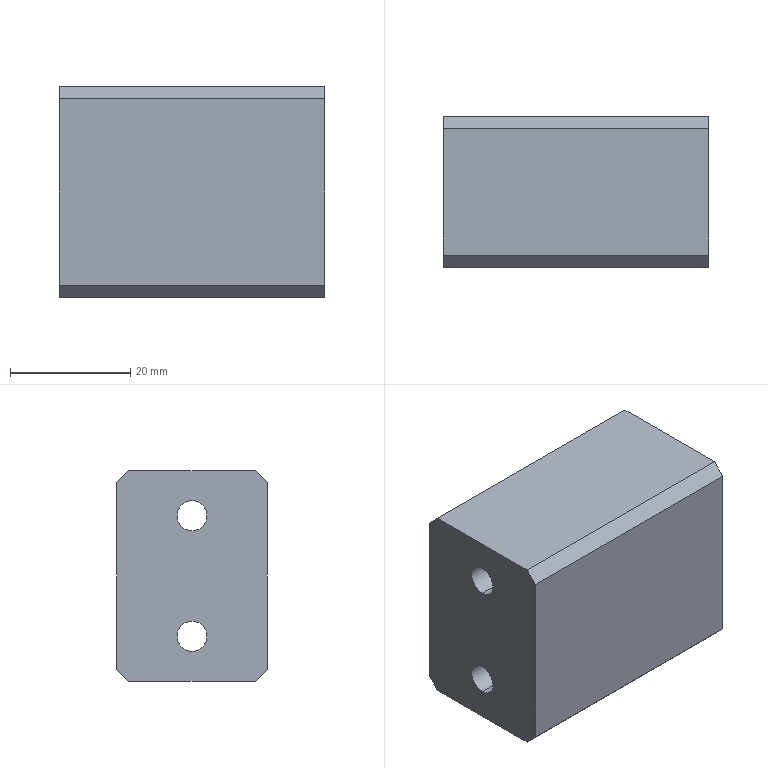Part | SolidWorks | features BaseBody 1 | 1 solid | 14 faces | box 44 x 25 x 35 mm | volume 36420 mm3 | plane 10 | cylinder 4 | commonest cylinder face diameters 5 x4
STEP:
#1=CARTESIAN_POINT('',(35.247,1517.,-337.));
#2=VERTEX_POINT('',#1);
#3=CARTESIAN_POINT('',(35.247,1517.,-332.));
#4=VERTEX_POINT('',#3);
#5=CARTESIAN_POINT('',(35.247,1517.,-334.5));
#6=DIRECTION('',(-1.,0.,0.));
#7=DIRECTION('',(0.,0.,-1.));
#8=AXIS2_PLACEMENT_3D('',#5,#6,#7);
#9=CIRCLE('',#8,2.5);
#10=EDGE_CURVE('',#2,#4,#9,.T.);
#11=ORIENTED_EDGE('',*,*,#10,.T.);
#12=CARTESIAN_POINT('',(79.247,1517.,-332.));
#13=VERTEX_POINT('',#12);
#14=CARTESIAN_POINT('',(79.247,1517.,-332.));
#15=DIRECTION('',(1.,0.,0.));
#16=VECTOR('',#15,1000.);
#17=LINE('',#14,#16);
#18=EDGE_CURVE('',#4,#13,#17,.T.);
#19=ORIENTED_EDGE('',*,*,#18,.T.);
#20=CARTESIAN_POINT('',(79.247,1517.,-337.));
#21=VERTEX_POINT('',#20);
#22=CARTESIAN_POINT('',(79.247,1517.,-334.5));
#23=DIRECTION('',(-1.,0.,0.));
#24=DIRECTION('',(0.,0.,-1.));
#25=AXIS2_PLACEMENT_3D('',#22,#23,#24);
#26=CIRCLE('',#25,2.5);
#27=EDGE_CURVE('',#21,#13,#26,.T.);
#28=ORIENTED_EDGE('',*,*,#27,.F.);
#29=CARTESIAN_POINT('',(79.247,1517.,-337.));
#30=DIRECTION('',(1.,0.,0.));
#31=VECTOR('',#30,1000.);
#32=LINE('',#29,#31);
#33=EDGE_CURVE('',#2,#21,#32,.T.);
#34=ORIENTED_EDGE('',*,*,#33,.F.);
#35=EDGE_LOOP('',(#11,#19,#28,#34));
#36=FACE_OUTER_BOUND('',#35,.T.);
#37=CARTESIAN_POINT('',(79.247,1517.,-334.5));
#38=DIRECTION('',(1.,0.,0.));
#39=DIRECTION('',(0.,0.,-1.));
#40=AXIS2_PLACEMENT_3D('',#37,#38,#39);
#41=CYLINDRICAL_SURFACE('',#40,2.5);
#42=ADVANCED_FACE('',(#36),#41,.F.);
#43=CARTESIAN_POINT('',(35.247,1517.,-357.));
#44=VERTEX_POINT('',#43);
#45=CARTESIAN_POINT('',(35.247,1517.,-352.));
#46=VERTEX_POINT('',#45);
#47=CARTESIAN_POINT('',(35.247,1517.,-354.5));
#48=DIRECTION('',(-1.,0.,0.));
#49=DIRECTION('',(0.,0.,-1.));
#50=AXIS2_PLACEMENT_3D('',#47,#48,#49);
#51=CIRCLE('',#50,2.5);
#52=EDGE_CURVE('',#44,#46,#51,.T.);
#53=ORIENTED_EDGE('',*,*,#52,.T.);
#54=CARTESIAN_POINT('',(79.247,1517.,-352.));
#55=VERTEX_POINT('',#54);
#56=CARTESIAN_POINT('',(79.247,1517.,-352.));
#57=DIRECTION('',(1.,0.,0.));
#58=VECTOR('',#57,1000.);
#59=LINE('',#56,#58);
#60=EDGE_CURVE('',#46,#55,#59,.T.);
#61=ORIENTED_EDGE('',*,*,#60,.T.);
#62=CARTESIAN_POINT('',(79.247,1517.,-357.));
#63=VERTEX_POINT('',#62);
#64=CARTESIAN_POINT('',(79.247,1517.,-354.5));
#65=DIRECTION('',(-1.,0.,0.));
#66=DIRECTION('',(0.,0.,-1.));
#67=AXIS2_PLACEMENT_3D('',#64,#65,#66);
#68=CIRCLE('',#67,2.5);
#69=EDGE_CURVE('',#63,#55,#68,.T.);
#70=ORIENTED_EDGE('',*,*,#69,.F.);
#71=CARTESIAN_POINT('',(79.247,1517.,-357.));
#72=DIRECTION('',(1.,0.,0.));
#73=VECTOR('',#72,1000.);
#74=LINE('',#71,#73);
#75=EDGE_CURVE('',#44,#63,#74,.T.);
#76=ORIENTED_EDGE('',*,*,#75,.F.);
#77=EDGE_LOOP('',(#53,#61,#70,#76));
#78=FACE_OUTER_BOUND('',#77,.T.);
#79=CARTESIAN_POINT('',(79.247,1517.,-354.5));
#80=DIRECTION('',(1.,0.,0.));
#81=DIRECTION('',(0.,0.,-1.));
#82=AXIS2_PLACEMENT_3D('',#79,#80,#81);
#83=CYLINDRICAL_SURFACE('',#82,2.5);
#84=ADVANCED_FACE('',(#78),#83,.F.);
#85=CARTESIAN_POINT('',(35.247,1529.5,-329.));
#86=VERTEX_POINT('',#85);
#87=CARTESIAN_POINT('',(35.247,1529.5,-360.));
#88=VERTEX_POINT('',#87);
#89=CARTESIAN_POINT('',(35.247,1529.5,-327.));
#90=DIRECTION('',(0.,0.,-1.));
#91=VECTOR('',#90,1000.);
#92=LINE('',#89,#91);
#93=EDGE_CURVE('',#86,#88,#92,.T.);
#94=ORIENTED_EDGE('',*,*,#93,.F.);
#95=CARTESIAN_POINT('',(79.247,1529.5,-329.));
#96=VERTEX_POINT('',#95);
#97=CARTESIAN_POINT('',(79.247,1529.5,-329.));
#98=DIRECTION('',(-1.,0.,0.));
#99=VECTOR('',#98,1000.);
#100=LINE('',#97,#99);
#101=EDGE_CURVE('',#96,#86,#100,.T.);
#102=ORIENTED_EDGE('',*,*,#101,.F.);
#103=CARTESIAN_POINT('',(79.247,1529.5,-360.));
#104=VERTEX_POINT('',#103);
#105=CARTESIAN_POINT('',(79.247,1529.5,-327.));
#106=DIRECTION('',(0.,0.,1.));
#107=VECTOR('',#106,1000.);
#108=LINE('',#105,#107);
#109=EDGE_CURVE('',#104,#96,#108,.T.);
#110=ORIENTED_EDGE('',*,*,#109,.F.);
#111=CARTESIAN_POINT('',(79.247,1529.5,-360.));
#112=DIRECTION('',(1.,0.,0.));
#113=VECTOR('',#112,1000.);
#114=LINE('',#111,#113);
#115=EDGE_CURVE('',#88,#104,#114,.T.);
#116=ORIENTED_EDGE('',*,*,#115,.F.);
#117=EDGE_LOOP('',(#94,#102,#110,#116));
#118=FACE_OUTER_BOUND('',#117,.T.);
#119=CARTESIAN_POINT('',(79.247,1529.5,-327.));
#120=DIRECTION('',(0.,-1.,0.));
#121=DIRECTION('',(0.,0.,-1.));
#122=AXIS2_PLACEMENT_3D('',#119,#120,#121);
#123=PLANE('',#122);
#124=ADVANCED_FACE('',(#118),#123,.F.);
#125=CARTESIAN_POINT('',(35.247,1527.5,-362.));
#126=VERTEX_POINT('',#125);
#127=CARTESIAN_POINT('',(35.247,1529.5,-360.));
#128=DIRECTION('',(0.,-0.7071,-0.7071));
#129=VECTOR('',#128,1000.);
#130=LINE('',#127,#129);
#131=EDGE_CURVE('',#88,#126,#130,.T.);
#132=ORIENTED_EDGE('',*,*,#131,.F.);
#133=ORIENTED_EDGE('',*,*,#115,.T.);
#134=CARTESIAN_POINT('',(79.247,1527.5,-362.));
#135=VERTEX_POINT('',#134);
#136=CARTESIAN_POINT('',(79.247,1529.5,-360.));
#137=DIRECTION('',(0.,0.7071,0.7071));
#138=VECTOR('',#137,1000.);
#139=LINE('',#136,#138);
#140=EDGE_CURVE('',#135,#104,#139,.T.);
#141=ORIENTED_EDGE('',*,*,#140,.F.);
#142=CARTESIAN_POINT('',(79.247,1527.5,-362.));
#143=DIRECTION('',(1.,0.,0.));
#144=VECTOR('',#143,1000.);
#145=LINE('',#142,#144);
#146=EDGE_CURVE('',#126,#135,#145,.T.);
#147=ORIENTED_EDGE('',*,*,#146,.F.);
#148=EDGE_LOOP('',(#132,#133,#141,#147));
#149=FACE_OUTER_BOUND('',#148,.T.);
#150=CARTESIAN_POINT('',(79.247,1529.5,-360.));
#151=DIRECTION('',(0.,-0.7071,0.7071));
#152=DIRECTION('',(0.,-0.7071,-0.7071));
#153=AXIS2_PLACEMENT_3D('',#150,#151,#152);
#154=PLANE('',#153);
#155=ADVANCED_FACE('',(#149),#154,.F.);
#156=ORIENTED_EDGE('',*,*,#10,.F.);
#157=CARTESIAN_POINT('',(35.247,1517.,-334.5));
#158=DIRECTION('',(-1.,0.,0.));
#159=DIRECTION('',(0.,0.,-1.));
#160=AXIS2_PLACEMENT_3D('',#157,#158,#159);
#161=CIRCLE('',#160,2.5);
#162=EDGE_CURVE('',#4,#2,#161,.T.);
#163=ORIENTED_EDGE('',*,*,#162,.F.);
#164=EDGE_LOOP('',(#156,#163));
#165=FACE_BOUND('',#164,.T.);
#166=ORIENTED_EDGE('',*,*,#52,.F.);
#167=CARTESIAN_POINT('',(35.247,1517.,-354.5));
#168=DIRECTION('',(-1.,0.,0.));
#169=DIRECTION('',(0.,0.,-1.));
#170=AXIS2_PLACEMENT_3D('',#167,#168,#169);
#171=CIRCLE('',#170,2.5);
#172=EDGE_CURVE('',#46,#44,#171,.T.);
#173=ORIENTED_EDGE('',*,*,#172,.F.);
#174=EDGE_LOOP('',(#166,#173));
#175=FACE_BOUND('',#174,.T.);
#176=CARTESIAN_POINT('',(35.247,1506.5,-362.));
#177=VERTEX_POINT('',#176);
#178=CARTESIAN_POINT('',(35.247,1517.,-362.));
#179=DIRECTION('',(0.,1.,0.));
#180=VECTOR('',#179,1000.);
#181=LINE('',#178,#180);
#182=EDGE_CURVE('',#177,#126,#181,.T.);
#183=ORIENTED_EDGE('',*,*,#182,.F.);
#184=CARTESIAN_POINT('',(35.247,1504.5,-360.));
#185=VERTEX_POINT('',#184);
#186=CARTESIAN_POINT('',(35.247,1504.5,-360.));
#187=DIRECTION('',(0.,0.7071,-0.7071));
#188=VECTOR('',#187,1000.);
#189=LINE('',#186,#188);
#190=EDGE_CURVE('',#185,#177,#189,.T.);
#191=ORIENTED_EDGE('',*,*,#190,.F.);
#192=CARTESIAN_POINT('',(35.247,1504.5,-329.));
#193=VERTEX_POINT('',#192);
#194=CARTESIAN_POINT('',(35.247,1504.5,-344.5));
#195=DIRECTION('',(0.,0.,-1.));
#196=VECTOR('',#195,1000.);
#197=LINE('',#194,#196);
#198=EDGE_CURVE('',#193,#185,#197,.T.);
#199=ORIENTED_EDGE('',*,*,#198,.F.);
#200=CARTESIAN_POINT('',(35.247,1506.5,-327.));
#201=VERTEX_POINT('',#200);
#202=CARTESIAN_POINT('',(35.247,1506.5,-327.));
#203=DIRECTION('',(0.,-0.7071,-0.7071));
#204=VECTOR('',#203,1000.);
#205=LINE('',#202,#204);
#206=EDGE_CURVE('',#201,#193,#205,.T.);
#207=ORIENTED_EDGE('',*,*,#206,.F.);
#208=CARTESIAN_POINT('',(35.247,1527.5,-327.));
#209=VERTEX_POINT('',#208);
#210=CARTESIAN_POINT('',(35.247,1517.,-327.));
#211=DIRECTION('',(0.,-1.,0.));
#212=VECTOR('',#211,1000.);
#213=LINE('',#210,#212);
#214=EDGE_CURVE('',#209,#201,#213,.T.);
#215=ORIENTED_EDGE('',*,*,#214,.F.);
#216=CARTESIAN_POINT('',(35.247,1529.5,-329.));
#217=DIRECTION('',(0.,-0.7071,0.7071));
#218=VECTOR('',#217,1000.);
#219=LINE('',#216,#218);
#220=EDGE_CURVE('',#86,#209,#219,.T.);
#221=ORIENTED_EDGE('',*,*,#220,.F.);
#222=ORIENTED_EDGE('',*,*,#93,.T.);
#223=ORIENTED_EDGE('',*,*,#131,.T.);
#224=EDGE_LOOP('',(#183,#191,#199,#207,#215,#221,#222,#223));
#225=FACE_OUTER_BOUND('',#224,.T.);
#226=CARTESIAN_POINT('',(35.247,1517.,-344.5));
#227=DIRECTION('',(1.,0.,0.));
#228=DIRECTION('',(0.,0.,-1.));
#229=AXIS2_PLACEMENT_3D('',#226,#227,#228);
#230=PLANE('',#229);
#231=ADVANCED_FACE('',(#165,#175,#225),#230,.F.);
#232=ORIENTED_EDGE('',*,*,#220,.T.);
#233=CARTESIAN_POINT('',(79.247,1527.5,-327.));
#234=VERTEX_POINT('',#233);
#235=CARTESIAN_POINT('',(79.247,1527.5,-327.));
#236=DIRECTION('',(-1.,0.,0.));
#237=VECTOR('',#236,1000.);
#238=LINE('',#235,#237);
#239=EDGE_CURVE('',#234,#209,#238,.T.);
#240=ORIENTED_EDGE('',*,*,#239,.F.);
#241=CARTESIAN_POINT('',(79.247,1527.5,-327.));
#242=DIRECTION('',(0.,-0.7071,0.7071));
#243=VECTOR('',#242,1000.);
#244=LINE('',#241,#243);
#245=EDGE_CURVE('',#96,#234,#244,.T.);
#246=ORIENTED_EDGE('',*,*,#245,.F.);
#247=ORIENTED_EDGE('',*,*,#101,.T.);
#248=EDGE_LOOP('',(#232,#240,#246,#247));
#249=FACE_OUTER_BOUND('',#248,.T.);
#250=CARTESIAN_POINT('',(79.247,1527.5,-327.));
#251=DIRECTION('',(0.,-0.7071,-0.7071));
#252=DIRECTION('',(0.,0.7071,-0.7071));
#253=AXIS2_PLACEMENT_3D('',#250,#251,#252);
#254=PLANE('',#253);
#255=ADVANCED_FACE('',(#249),#254,.F.);
#256=ORIENTED_EDGE('',*,*,#27,.T.);
#257=CARTESIAN_POINT('',(79.247,1517.,-334.5));
#258=DIRECTION('',(-1.,0.,0.));
#259=DIRECTION('',(0.,0.,-1.));
#260=AXIS2_PLACEMENT_3D('',#257,#258,#259);
#261=CIRCLE('',#260,2.5);
#262=EDGE_CURVE('',#13,#21,#261,.T.);
#263=ORIENTED_EDGE('',*,*,#262,.T.);
#264=EDGE_LOOP('',(#256,#263));
#265=FACE_BOUND('',#264,.T.);
#266=ORIENTED_EDGE('',*,*,#69,.T.);
#267=CARTESIAN_POINT('',(79.247,1517.,-354.5));
#268=DIRECTION('',(-1.,0.,0.));
#269=DIRECTION('',(0.,0.,-1.));
#270=AXIS2_PLACEMENT_3D('',#267,#268,#269);
#271=CIRCLE('',#270,2.5);
#272=EDGE_CURVE('',#55,#63,#271,.T.);
#273=ORIENTED_EDGE('',*,*,#272,.T.);
#274=EDGE_LOOP('',(#266,#273));
#275=FACE_BOUND('',#274,.T.);
#276=CARTESIAN_POINT('',(79.247,1504.5,-360.));
#277=VERTEX_POINT('',#276);
#278=CARTESIAN_POINT('',(79.247,1506.5,-362.));
#279=VERTEX_POINT('',#278);
#280=CARTESIAN_POINT('',(79.247,1504.5,-360.));
#281=DIRECTION('',(0.,0.7071,-0.7071));
#282=VECTOR('',#281,1000.);
#283=LINE('',#280,#282);
#284=EDGE_CURVE('',#277,#279,#283,.T.);
#285=ORIENTED_EDGE('',*,*,#284,.T.);
#286=CARTESIAN_POINT('',(79.247,1517.,-362.));
#287=DIRECTION('',(0.,1.,0.));
#288=VECTOR('',#287,1000.);
#289=LINE('',#286,#288);
#290=EDGE_CURVE('',#279,#135,#289,.T.);
#291=ORIENTED_EDGE('',*,*,#290,.T.);
#292=ORIENTED_EDGE('',*,*,#140,.T.);
#293=ORIENTED_EDGE('',*,*,#109,.T.);
#294=ORIENTED_EDGE('',*,*,#245,.T.);
#295=CARTESIAN_POINT('',(79.247,1506.5,-327.));
#296=VERTEX_POINT('',#295);
#297=CARTESIAN_POINT('',(79.247,1517.,-327.));
#298=DIRECTION('',(0.,-1.,0.));
#299=VECTOR('',#298,1000.);
#300=LINE('',#297,#299);
#301=EDGE_CURVE('',#234,#296,#300,.T.);
#302=ORIENTED_EDGE('',*,*,#301,.T.);
#303=CARTESIAN_POINT('',(79.247,1504.5,-329.));
#304=VERTEX_POINT('',#303);
#305=CARTESIAN_POINT('',(79.247,1506.5,-327.));
#306=DIRECTION('',(0.,-0.7071,-0.7071));
#307=VECTOR('',#306,1000.);
#308=LINE('',#305,#307);
#309=EDGE_CURVE('',#296,#304,#308,.T.);
#310=ORIENTED_EDGE('',*,*,#309,.T.);
#311=CARTESIAN_POINT('',(79.247,1504.5,-344.5));
#312=DIRECTION('',(0.,0.,-1.));
#313=VECTOR('',#312,1000.);
#314=LINE('',#311,#313);
#315=EDGE_CURVE('',#304,#277,#314,.T.);
#316=ORIENTED_EDGE('',*,*,#315,.T.);
#317=EDGE_LOOP('',(#285,#291,#292,#293,#294,#302,#310,#316));
#318=FACE_OUTER_BOUND('',#317,.T.);
#319=CARTESIAN_POINT('',(79.247,1517.,-344.5));
#320=DIRECTION('',(1.,0.,0.));
#321=DIRECTION('',(0.,0.,-1.));
#322=AXIS2_PLACEMENT_3D('',#319,#320,#321);
#323=PLANE('',#322);
#324=ADVANCED_FACE('',(#265,#275,#318),#323,.T.);
#325=ORIENTED_EDGE('',*,*,#290,.F.);
#326=CARTESIAN_POINT('',(79.247,1506.5,-362.));
#327=DIRECTION('',(1.,0.,0.));
#328=VECTOR('',#327,1000.);
#329=LINE('',#326,#328);
#330=EDGE_CURVE('',#177,#279,#329,.T.);
#331=ORIENTED_EDGE('',*,*,#330,.F.);
#332=ORIENTED_EDGE('',*,*,#182,.T.);
#333=ORIENTED_EDGE('',*,*,#146,.T.);
#334=EDGE_LOOP('',(#325,#331,#332,#333));
#335=FACE_OUTER_BOUND('',#334,.T.);
#336=CARTESIAN_POINT('',(79.247,1504.5,-362.));
#337=DIRECTION('',(0.,0.,1.));
#338=DIRECTION('',(1.,0.,0.));
#339=AXIS2_PLACEMENT_3D('',#336,#337,#338);
#340=PLANE('',#339);
#341=ADVANCED_FACE('',(#335),#340,.F.);
#342=ORIENTED_EDGE('',*,*,#18,.F.);
#343=ORIENTED_EDGE('',*,*,#162,.T.);
#344=ORIENTED_EDGE('',*,*,#33,.T.);
#345=ORIENTED_EDGE('',*,*,#262,.F.);
#346=EDGE_LOOP('',(#342,#343,#344,#345));
#347=FACE_OUTER_BOUND('',#346,.T.);
#348=CARTESIAN_POINT('',(79.247,1517.,-334.5));
#349=DIRECTION('',(1.,0.,0.));
#350=DIRECTION('',(0.,0.,-1.));
#351=AXIS2_PLACEMENT_3D('',#348,#349,#350);
#352=CYLINDRICAL_SURFACE('',#351,2.5);
#353=ADVANCED_FACE('',(#347),#352,.F.);
#354=ORIENTED_EDGE('',*,*,#60,.F.);
#355=ORIENTED_EDGE('',*,*,#172,.T.);
#356=ORIENTED_EDGE('',*,*,#75,.T.);
#357=ORIENTED_EDGE('',*,*,#272,.F.);
#358=EDGE_LOOP('',(#354,#355,#356,#357));
#359=FACE_OUTER_BOUND('',#358,.T.);
#360=CARTESIAN_POINT('',(79.247,1517.,-354.5));
#361=DIRECTION('',(1.,0.,0.));
#362=DIRECTION('',(0.,0.,-1.));
#363=AXIS2_PLACEMENT_3D('',#360,#361,#362);
#364=CYLINDRICAL_SURFACE('',#363,2.5);
#365=ADVANCED_FACE('',(#359),#364,.F.);
#366=ORIENTED_EDGE('',*,*,#190,.T.);
#367=ORIENTED_EDGE('',*,*,#330,.T.);
#368=ORIENTED_EDGE('',*,*,#284,.F.);
#369=CARTESIAN_POINT('',(79.247,1504.5,-360.));
#370=DIRECTION('',(1.,0.,0.));
#371=VECTOR('',#370,1000.);
#372=LINE('',#369,#371);
#373=EDGE_CURVE('',#185,#277,#372,.T.);
#374=ORIENTED_EDGE('',*,*,#373,.F.);
#375=EDGE_LOOP('',(#366,#367,#368,#374));
#376=FACE_OUTER_BOUND('',#375,.T.);
#377=CARTESIAN_POINT('',(79.247,1506.5,-362.));
#378=DIRECTION('',(0.,0.7071,0.7071));
#379=DIRECTION('',(0.,-0.7071,0.7071));
#380=AXIS2_PLACEMENT_3D('',#377,#378,#379);
#381=PLANE('',#380);
#382=ADVANCED_FACE('',(#376),#381,.F.);
#383=ORIENTED_EDGE('',*,*,#315,.F.);
#384=CARTESIAN_POINT('',(79.247,1504.5,-329.));
#385=DIRECTION('',(1.,0.,0.));
#386=VECTOR('',#385,1000.);
#387=LINE('',#384,#386);
#388=EDGE_CURVE('',#193,#304,#387,.T.);
#389=ORIENTED_EDGE('',*,*,#388,.F.);
#390=ORIENTED_EDGE('',*,*,#198,.T.);
#391=ORIENTED_EDGE('',*,*,#373,.T.);
#392=EDGE_LOOP('',(#383,#389,#390,#391));
#393=FACE_OUTER_BOUND('',#392,.T.);
#394=CARTESIAN_POINT('',(79.247,1504.5,-327.));
#395=DIRECTION('',(0.,1.,0.));
#396=DIRECTION('',(0.,0.,1.));
#397=AXIS2_PLACEMENT_3D('',#394,#395,#396);
#398=PLANE('',#397);
#399=ADVANCED_FACE('',(#393),#398,.F.);
#400=ORIENTED_EDGE('',*,*,#206,.T.);
#401=ORIENTED_EDGE('',*,*,#388,.T.);
#402=ORIENTED_EDGE('',*,*,#309,.F.);
#403=CARTESIAN_POINT('',(79.247,1506.5,-327.));
#404=DIRECTION('',(1.,0.,0.));
#405=VECTOR('',#404,1000.);
#406=LINE('',#403,#405);
#407=EDGE_CURVE('',#201,#296,#406,.T.);
#408=ORIENTED_EDGE('',*,*,#407,.F.);
#409=EDGE_LOOP('',(#400,#401,#402,#408));
#410=FACE_OUTER_BOUND('',#409,.T.);
#411=CARTESIAN_POINT('',(79.247,1504.5,-329.));
#412=DIRECTION('',(0.,0.7071,-0.7071));
#413=DIRECTION('',(0.,0.7071,0.7071));
#414=AXIS2_PLACEMENT_3D('',#411,#412,#413);
#415=PLANE('',#414);
#416=ADVANCED_FACE('',(#410),#415,.F.);
#417=ORIENTED_EDGE('',*,*,#214,.T.);
#418=ORIENTED_EDGE('',*,*,#407,.T.);
#419=ORIENTED_EDGE('',*,*,#301,.F.);
#420=ORIENTED_EDGE('',*,*,#239,.T.);
#421=EDGE_LOOP('',(#417,#418,#419,#420));
#422=FACE_OUTER_BOUND('',#421,.T.);
#423=CARTESIAN_POINT('',(79.247,1504.5,-327.));
#424=DIRECTION('',(0.,0.,-1.));
#425=DIRECTION('',(-1.,0.,0.));
#426=AXIS2_PLACEMENT_3D('',#423,#424,#425);
#427=PLANE('',#426);
#428=ADVANCED_FACE('',(#422),#427,.F.);
#429=CLOSED_SHELL('',(#42,#84,#124,#155,#231,#255,#324,#341,#353,#365,#382,#399,#416,#428));
#430=MANIFOLD_SOLID_BREP('',#429);
#431=CARTESIAN_POINT('',(0.,0.,0.));
#432=DIRECTION('',(0.,0.,1.));
#433=DIRECTION('',(1.,0.,0.));
#434=AXIS2_PLACEMENT_3D('',#431,#432,#433);
#435=(LENGTH_UNIT()NAMED_UNIT(*)SI_UNIT(.MILLI.,.METRE.));
#436=UNCERTAINTY_MEASURE_WITH_UNIT(LENGTH_MEASURE(0.00001),#435,'','');
#437=(NAMED_UNIT(*)PLANE_ANGLE_UNIT()SI_UNIT($,.RADIAN.));
#438=(NAMED_UNIT(*)SI_UNIT($,.STERADIAN.)SOLID_ANGLE_UNIT());
#439=(GEOMETRIC_REPRESENTATION_CONTEXT(3)GLOBAL_UNCERTAINTY_ASSIGNED_CONTEXT((#436))GLOBAL_UNIT_ASSIGNED_CONTEXT((#435,#437,#438))REPRESENTATION_CONTEXT('',''));
#440=ADVANCED_BREP_SHAPE_REPRESENTATION('',(#430,#434),#439);